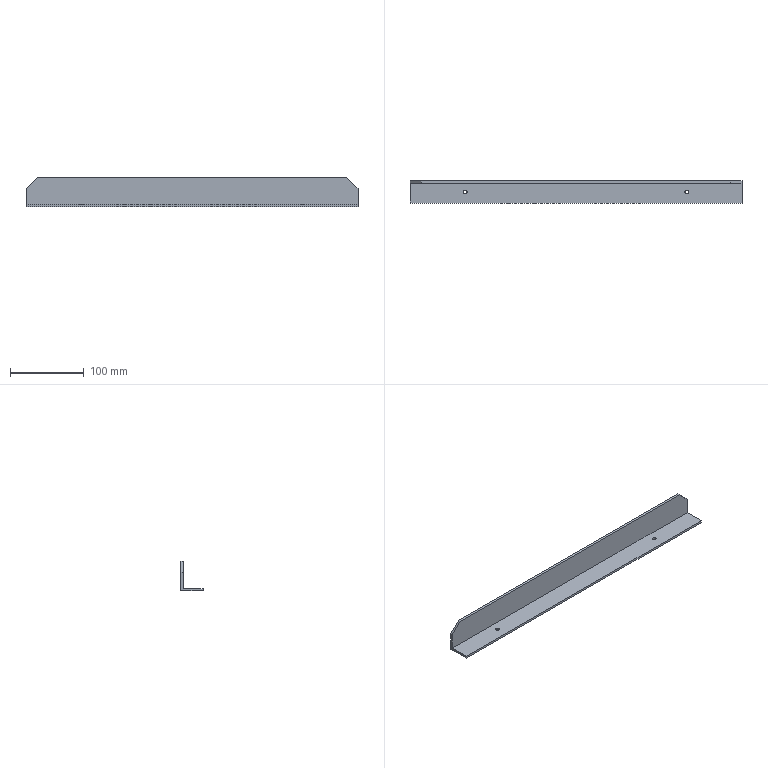Part | STEP file | Electrical cabinet partition strip | 1 solid | 14 faces | box 450 x 30 x 40 mm | volume 89657 mm3 | plane 10 | cylinder 4 | commonest cylinder face diameters 5 x4
STEP:
#1=CARTESIAN_POINT('',(0.,0.,0.));
#2=DIRECTION('',(0.,0.,1.));
#3=DIRECTION('',(1.,0.,0.));
#4=AXIS2_PLACEMENT_3D('',#1,#2,#3);
#5=CARTESIAN_POINT('',(77.5,30.066,-52.253));
#6=VERTEX_POINT('',#5);
#7=CARTESIAN_POINT('',(77.5,30.066,-49.253));
#8=VERTEX_POINT('',#7);
#9=CARTESIAN_POINT('',(77.5,30.066,-499.253));
#10=DIRECTION('',(0.,0.,1.));
#11=VECTOR('',#10,1.);
#12=LINE('',#9,#11);
#13=CARTESIAN_POINT('',(75.,30.066,-499.253));
#14=DIRECTION('',(0.,0.,1.));
#15=DIRECTION('',(1.,0.,0.));
#16=AXIS2_PLACEMENT_3D('',#13,#14,#15);
#17=CYLINDRICAL_SURFACE('',#16,2.5);
#18=CARTESIAN_POINT('',(6.283,0.));
#19=DIRECTION('',(0.,1.));
#20=VECTOR('',#19,1.);
#21=LINE('',#18,#20);
#22=(GEOMETRIC_REPRESENTATION_CONTEXT(2)PARAMETRIC_REPRESENTATION_CONTEXT()REPRESENTATION_CONTEXT('',''));
#23=DEFINITIONAL_REPRESENTATION('',(#21),#22);
#24=PCURVE('',#17,#23);
#25=CARTESIAN_POINT('',(75.,30.066,-499.253));
#26=DIRECTION('',(0.,0.,1.));
#27=DIRECTION('',(1.,0.,0.));
#28=AXIS2_PLACEMENT_3D('',#25,#26,#27);
#29=CYLINDRICAL_SURFACE('',#28,2.5);
#30=CARTESIAN_POINT('',(0.,0.));
#31=DIRECTION('',(0.,1.));
#32=VECTOR('',#31,1.);
#33=LINE('',#30,#32);
#34=(GEOMETRIC_REPRESENTATION_CONTEXT(2)PARAMETRIC_REPRESENTATION_CONTEXT()REPRESENTATION_CONTEXT('',''));
#35=DEFINITIONAL_REPRESENTATION('',(#33),#34);
#36=PCURVE('',#29,#35);
#37=SURFACE_CURVE('',#12,(#24,#36),.PCURVE_S1.);
#38=EDGE_CURVE('',#6,#8,#37,.T.);
#39=ORIENTED_EDGE('',*,*,#38,.T.);
#40=CARTESIAN_POINT('',(72.5,30.066,-49.253));
#41=VERTEX_POINT('',#40);
#42=CARTESIAN_POINT('',(75.,30.066,-49.253));
#43=DIRECTION('',(0.,0.,1.));
#44=DIRECTION('',(1.,0.,0.));
#45=AXIS2_PLACEMENT_3D('',#42,#43,#44);
#46=CIRCLE('',#45,2.5);
#47=CARTESIAN_POINT('',(0.,450.));
#48=DIRECTION('',(1.,0.));
#49=VECTOR('',#48,1.);
#50=LINE('',#47,#49);
#51=(GEOMETRIC_REPRESENTATION_CONTEXT(2)PARAMETRIC_REPRESENTATION_CONTEXT()REPRESENTATION_CONTEXT('',''));
#52=DEFINITIONAL_REPRESENTATION('',(#50),#51);
#53=PCURVE('',#17,#52);
#54=CARTESIAN_POINT('',(450.,42.066,-49.253));
#55=DIRECTION('',(0.,0.,-1.));
#56=DIRECTION('',(0.,1.,0.));
#57=AXIS2_PLACEMENT_3D('',#54,#55,#56);
#58=PLANE('',#57);
#59=CARTESIAN_POINT('',(-12.,-372.5));
#60=CARTESIAN_POINT('',(-7.67,-372.5));
#61=CARTESIAN_POINT('',(-9.835,-376.25));
#62=CARTESIAN_POINT('',(-12.,-380.));
#63=CARTESIAN_POINT('',(-14.165,-376.25));
#64=CARTESIAN_POINT('',(-16.33,-372.5));
#65=CARTESIAN_POINT('',(-12.,-372.5));
#66=(BOUNDED_CURVE()B_SPLINE_CURVE(2,(#59,#60,#61,#62,#63,#64,#65),.UNSPECIFIED.,.T.,.F.)B_SPLINE_CURVE_WITH_KNOTS((1,2,2,2,2,1),(-2.094,0.,2.094,4.189,6.283,8.378),.UNSPECIFIED.)CURVE()GEOMETRIC_REPRESENTATION_ITEM()RATIONAL_B_SPLINE_CURVE((1.,0.5,1.,0.5,1.,0.5,1.))REPRESENTATION_ITEM(''));
#67=(GEOMETRIC_REPRESENTATION_CONTEXT(2)PARAMETRIC_REPRESENTATION_CONTEXT()REPRESENTATION_CONTEXT('',''));
#68=DEFINITIONAL_REPRESENTATION('',(#66),#67);
#69=PCURVE('',#58,#68);
#70=SURFACE_CURVE('',#46,(#53,#69),.PCURVE_S1.);
#71=EDGE_CURVE('',#41,#8,#70,.T.);
#72=ORIENTED_EDGE('',*,*,#71,.F.);
#73=CARTESIAN_POINT('',(72.5,30.066,-52.253));
#74=VERTEX_POINT('',#73);
#75=CARTESIAN_POINT('',(72.5,30.066,-499.253));
#76=DIRECTION('',(0.,0.,1.));
#77=VECTOR('',#76,1.);
#78=LINE('',#75,#77);
#79=CARTESIAN_POINT('',(3.142,0.));
#80=DIRECTION('',(0.,1.));
#81=VECTOR('',#80,1.);
#82=LINE('',#79,#81);
#83=(GEOMETRIC_REPRESENTATION_CONTEXT(2)PARAMETRIC_REPRESENTATION_CONTEXT()REPRESENTATION_CONTEXT('',''));
#84=DEFINITIONAL_REPRESENTATION('',(#82),#83);
#85=PCURVE('',#17,#84);
#86=CARTESIAN_POINT('',(3.142,0.));
#87=DIRECTION('',(0.,1.));
#88=VECTOR('',#87,1.);
#89=LINE('',#86,#88);
#90=(GEOMETRIC_REPRESENTATION_CONTEXT(2)PARAMETRIC_REPRESENTATION_CONTEXT()REPRESENTATION_CONTEXT('',''));
#91=DEFINITIONAL_REPRESENTATION('',(#89),#90);
#92=PCURVE('',#29,#91);
#93=SURFACE_CURVE('',#78,(#85,#92),.PCURVE_S1.);
#94=EDGE_CURVE('',#74,#41,#93,.T.);
#95=ORIENTED_EDGE('',*,*,#94,.F.);
#96=CARTESIAN_POINT('',(75.,30.066,-52.253));
#97=DIRECTION('',(0.,0.,1.));
#98=DIRECTION('',(0.,-1.,0.));
#99=AXIS2_PLACEMENT_3D('',#96,#97,#98);
#100=CIRCLE('',#99,2.5);
#101=CARTESIAN_POINT('',(-1.571,447.));
#102=DIRECTION('',(1.,0.));
#103=VECTOR('',#102,1.);
#104=LINE('',#101,#103);
#105=(GEOMETRIC_REPRESENTATION_CONTEXT(2)PARAMETRIC_REPRESENTATION_CONTEXT()REPRESENTATION_CONTEXT('',''));
#106=DEFINITIONAL_REPRESENTATION('',(#104),#105);
#107=PCURVE('',#17,#106);
#108=CARTESIAN_POINT('',(450.,45.066,-52.253));
#109=DIRECTION('',(0.,0.,1.));
#110=DIRECTION('',(0.,-1.,0.));
#111=AXIS2_PLACEMENT_3D('',#108,#109,#110);
#112=PLANE('',#111);
#113=CARTESIAN_POINT('',(15.,-375.));
#114=DIRECTION('',(1.,0.));
#115=AXIS2_PLACEMENT_2D('',#113,#114);
#116=CIRCLE('',#115,2.5);
#117=(GEOMETRIC_REPRESENTATION_CONTEXT(2)PARAMETRIC_REPRESENTATION_CONTEXT()REPRESENTATION_CONTEXT('',''));
#118=DEFINITIONAL_REPRESENTATION('',(#116),#117);
#119=PCURVE('',#112,#118);
#120=SURFACE_CURVE('',#100,(#107,#119),.PCURVE_S1.);
#121=EDGE_CURVE('',#74,#6,#120,.T.);
#122=ORIENTED_EDGE('',*,*,#121,.T.);
#123=EDGE_LOOP('',(#39,#72,#95,#122));
#124=FACE_BOUND('',#123,.F.);
#125=ADVANCED_FACE('',(#124),#17,.F.);
#126=CARTESIAN_POINT('',(377.5,30.066,-52.253));
#127=VERTEX_POINT('',#126);
#128=CARTESIAN_POINT('',(377.5,30.066,-49.253));
#129=VERTEX_POINT('',#128);
#130=CARTESIAN_POINT('',(377.5,30.066,-499.253));
#131=DIRECTION('',(0.,0.,1.));
#132=VECTOR('',#131,1.);
#133=LINE('',#130,#132);
#134=CARTESIAN_POINT('',(375.,30.066,-499.253));
#135=DIRECTION('',(0.,0.,1.));
#136=DIRECTION('',(1.,0.,0.));
#137=AXIS2_PLACEMENT_3D('',#134,#135,#136);
#138=CYLINDRICAL_SURFACE('',#137,2.5);
#139=CARTESIAN_POINT('',(6.283,0.));
#140=DIRECTION('',(0.,1.));
#141=VECTOR('',#140,1.);
#142=LINE('',#139,#141);
#143=(GEOMETRIC_REPRESENTATION_CONTEXT(2)PARAMETRIC_REPRESENTATION_CONTEXT()REPRESENTATION_CONTEXT('',''));
#144=DEFINITIONAL_REPRESENTATION('',(#142),#143);
#145=PCURVE('',#138,#144);
#146=CARTESIAN_POINT('',(375.,30.066,-499.253));
#147=DIRECTION('',(0.,0.,1.));
#148=DIRECTION('',(1.,0.,0.));
#149=AXIS2_PLACEMENT_3D('',#146,#147,#148);
#150=CYLINDRICAL_SURFACE('',#149,2.5);
#151=CARTESIAN_POINT('',(0.,0.));
#152=DIRECTION('',(0.,1.));
#153=VECTOR('',#152,1.);
#154=LINE('',#151,#153);
#155=(GEOMETRIC_REPRESENTATION_CONTEXT(2)PARAMETRIC_REPRESENTATION_CONTEXT()REPRESENTATION_CONTEXT('',''));
#156=DEFINITIONAL_REPRESENTATION('',(#154),#155);
#157=PCURVE('',#150,#156);
#158=SURFACE_CURVE('',#133,(#145,#157),.PCURVE_S1.);
#159=EDGE_CURVE('',#127,#129,#158,.T.);
#160=ORIENTED_EDGE('',*,*,#159,.T.);
#161=CARTESIAN_POINT('',(372.5,30.066,-49.253));
#162=VERTEX_POINT('',#161);
#163=CARTESIAN_POINT('',(375.,30.066,-49.253));
#164=DIRECTION('',(0.,0.,1.));
#165=DIRECTION('',(1.,0.,0.));
#166=AXIS2_PLACEMENT_3D('',#163,#164,#165);
#167=CIRCLE('',#166,2.5);
#168=CARTESIAN_POINT('',(0.,450.));
#169=DIRECTION('',(1.,0.));
#170=VECTOR('',#169,1.);
#171=LINE('',#168,#170);
#172=(GEOMETRIC_REPRESENTATION_CONTEXT(2)PARAMETRIC_REPRESENTATION_CONTEXT()REPRESENTATION_CONTEXT('',''));
#173=DEFINITIONAL_REPRESENTATION('',(#171),#172);
#174=PCURVE('',#138,#173);
#175=CARTESIAN_POINT('',(-12.,-72.5));
#176=CARTESIAN_POINT('',(-7.67,-72.5));
#177=CARTESIAN_POINT('',(-9.835,-76.25));
#178=CARTESIAN_POINT('',(-12.,-80.));
#179=CARTESIAN_POINT('',(-14.165,-76.25));
#180=CARTESIAN_POINT('',(-16.33,-72.5));
#181=CARTESIAN_POINT('',(-12.,-72.5));
#182=(BOUNDED_CURVE()B_SPLINE_CURVE(2,(#175,#176,#177,#178,#179,#180,#181),.UNSPECIFIED.,.T.,.F.)B_SPLINE_CURVE_WITH_KNOTS((1,2,2,2,2,1),(-2.094,0.,2.094,4.189,6.283,8.378),.UNSPECIFIED.)CURVE()GEOMETRIC_REPRESENTATION_ITEM()RATIONAL_B_SPLINE_CURVE((1.,0.5,1.,0.5,1.,0.5,1.))REPRESENTATION_ITEM(''));
#183=(GEOMETRIC_REPRESENTATION_CONTEXT(2)PARAMETRIC_REPRESENTATION_CONTEXT()REPRESENTATION_CONTEXT('',''));
#184=DEFINITIONAL_REPRESENTATION('',(#182),#183);
#185=PCURVE('',#58,#184);
#186=SURFACE_CURVE('',#167,(#174,#185),.PCURVE_S1.);
#187=EDGE_CURVE('',#162,#129,#186,.T.);
#188=ORIENTED_EDGE('',*,*,#187,.F.);
#189=CARTESIAN_POINT('',(372.5,30.066,-52.253));
#190=VERTEX_POINT('',#189);
#191=CARTESIAN_POINT('',(372.5,30.066,-499.253));
#192=DIRECTION('',(0.,0.,1.));
#193=VECTOR('',#192,1.);
#194=LINE('',#191,#193);
#195=CARTESIAN_POINT('',(3.142,0.));
#196=DIRECTION('',(0.,1.));
#197=VECTOR('',#196,1.);
#198=LINE('',#195,#197);
#199=(GEOMETRIC_REPRESENTATION_CONTEXT(2)PARAMETRIC_REPRESENTATION_CONTEXT()REPRESENTATION_CONTEXT('',''));
#200=DEFINITIONAL_REPRESENTATION('',(#198),#199);
#201=PCURVE('',#138,#200);
#202=CARTESIAN_POINT('',(3.142,0.));
#203=DIRECTION('',(0.,1.));
#204=VECTOR('',#203,1.);
#205=LINE('',#202,#204);
#206=(GEOMETRIC_REPRESENTATION_CONTEXT(2)PARAMETRIC_REPRESENTATION_CONTEXT()REPRESENTATION_CONTEXT('',''));
#207=DEFINITIONAL_REPRESENTATION('',(#205),#206);
#208=PCURVE('',#150,#207);
#209=SURFACE_CURVE('',#194,(#201,#208),.PCURVE_S1.);
#210=EDGE_CURVE('',#190,#162,#209,.T.);
#211=ORIENTED_EDGE('',*,*,#210,.F.);
#212=CARTESIAN_POINT('',(375.,30.066,-52.253));
#213=DIRECTION('',(0.,0.,1.));
#214=DIRECTION('',(0.,-1.,0.));
#215=AXIS2_PLACEMENT_3D('',#212,#213,#214);
#216=CIRCLE('',#215,2.5);
#217=CARTESIAN_POINT('',(-1.571,447.));
#218=DIRECTION('',(1.,0.));
#219=VECTOR('',#218,1.);
#220=LINE('',#217,#219);
#221=(GEOMETRIC_REPRESENTATION_CONTEXT(2)PARAMETRIC_REPRESENTATION_CONTEXT()REPRESENTATION_CONTEXT('',''));
#222=DEFINITIONAL_REPRESENTATION('',(#220),#221);
#223=PCURVE('',#138,#222);
#224=CARTESIAN_POINT('',(15.,-75.));
#225=DIRECTION('',(1.,0.));
#226=AXIS2_PLACEMENT_2D('',#224,#225);
#227=CIRCLE('',#226,2.5);
#228=(GEOMETRIC_REPRESENTATION_CONTEXT(2)PARAMETRIC_REPRESENTATION_CONTEXT()REPRESENTATION_CONTEXT('',''));
#229=DEFINITIONAL_REPRESENTATION('',(#227),#228);
#230=PCURVE('',#112,#229);
#231=SURFACE_CURVE('',#216,(#223,#230),.PCURVE_S1.);
#232=EDGE_CURVE('',#190,#127,#231,.T.);
#233=ORIENTED_EDGE('',*,*,#232,.T.);
#234=EDGE_LOOP('',(#160,#188,#211,#233));
#235=FACE_BOUND('',#234,.F.);
#236=ADVANCED_FACE('',(#235),#138,.F.);
#237=CARTESIAN_POINT('',(435.,42.066,-12.253));
#238=VERTEX_POINT('',#237);
#239=CARTESIAN_POINT('',(15.,42.066,-12.253));
#240=VERTEX_POINT('',#239);
#241=CARTESIAN_POINT('',(450.,42.066,-12.253));
#242=DIRECTION('',(-1.,0.,0.));
#243=VECTOR('',#242,1.);
#244=LINE('',#241,#243);
#245=CARTESIAN_POINT('',(450.,42.066,-12.253));
#246=DIRECTION('',(0.,0.,-1.));
#247=DIRECTION('',(-1.,0.,0.));
#248=AXIS2_PLACEMENT_3D('',#245,#246,#247);
#249=PLANE('',#248);
#250=CARTESIAN_POINT('',(0.,0.));
#251=DIRECTION('',(1.,0.));
#252=VECTOR('',#251,1.);
#253=LINE('',#250,#252);
#254=(GEOMETRIC_REPRESENTATION_CONTEXT(2)PARAMETRIC_REPRESENTATION_CONTEXT()REPRESENTATION_CONTEXT('',''));
#255=DEFINITIONAL_REPRESENTATION('',(#253),#254);
#256=PCURVE('',#249,#255);
#257=CARTESIAN_POINT('',(450.,42.066,-12.253));
#258=DIRECTION('',(0.,1.,0.));
#259=DIRECTION('',(0.,0.,1.));
#260=AXIS2_PLACEMENT_3D('',#257,#258,#259);
#261=PLANE('',#260);
#262=CARTESIAN_POINT('',(0.,0.));
#263=DIRECTION('',(0.,-1.));
#264=VECTOR('',#263,1.);
#265=LINE('',#262,#264);
#266=(GEOMETRIC_REPRESENTATION_CONTEXT(2)PARAMETRIC_REPRESENTATION_CONTEXT()REPRESENTATION_CONTEXT('',''));
#267=DEFINITIONAL_REPRESENTATION('',(#265),#266);
#268=PCURVE('',#261,#267);
#269=SURFACE_CURVE('',#244,(#256,#268),.PCURVE_S1.);
#270=EDGE_CURVE('',#238,#240,#269,.T.);
#271=ORIENTED_EDGE('',*,*,#270,.F.);
#272=CARTESIAN_POINT('',(435.,45.066,-12.253));
#273=VERTEX_POINT('',#272);
#274=CARTESIAN_POINT('',(435.,42.066,-12.253));
#275=DIRECTION('',(0.,1.,0.));
#276=VECTOR('',#275,1.);
#277=LINE('',#274,#276);
#278=CARTESIAN_POINT('',(15.,0.));
#279=DIRECTION('',(0.,1.));
#280=VECTOR('',#279,1.);
#281=LINE('',#278,#280);
#282=(GEOMETRIC_REPRESENTATION_CONTEXT(2)PARAMETRIC_REPRESENTATION_CONTEXT()REPRESENTATION_CONTEXT('',''));
#283=DEFINITIONAL_REPRESENTATION('',(#281),#282);
#284=PCURVE('',#249,#283);
#285=CARTESIAN_POINT('',(450.,0.,-27.253));
#286=DIRECTION('',(-0.7071,0.,-0.7071));
#287=DIRECTION('',(0.,-1.,0.));
#288=AXIS2_PLACEMENT_3D('',#285,#286,#287);
#289=PLANE('',#288);
#290=CARTESIAN_POINT('',(-42.066,21.213));
#291=DIRECTION('',(-1.,0.));
#292=VECTOR('',#291,1.);
#293=LINE('',#290,#292);
#294=(GEOMETRIC_REPRESENTATION_CONTEXT(2)PARAMETRIC_REPRESENTATION_CONTEXT()REPRESENTATION_CONTEXT('',''));
#295=DEFINITIONAL_REPRESENTATION('',(#293),#294);
#296=PCURVE('',#289,#295);
#297=SURFACE_CURVE('',#277,(#284,#296),.PCURVE_S1.);
#298=EDGE_CURVE('',#238,#273,#297,.T.);
#299=ORIENTED_EDGE('',*,*,#298,.T.);
#300=CARTESIAN_POINT('',(15.,45.066,-12.253));
#301=VERTEX_POINT('',#300);
#302=CARTESIAN_POINT('',(450.,45.066,-12.253));
#303=DIRECTION('',(-1.,0.,0.));
#304=VECTOR('',#303,1.);
#305=LINE('',#302,#304);
#306=CARTESIAN_POINT('',(0.,3.));
#307=DIRECTION('',(1.,0.));
#308=VECTOR('',#307,1.);
#309=LINE('',#306,#308);
#310=(GEOMETRIC_REPRESENTATION_CONTEXT(2)PARAMETRIC_REPRESENTATION_CONTEXT()REPRESENTATION_CONTEXT('',''));
#311=DEFINITIONAL_REPRESENTATION('',(#309),#310);
#312=PCURVE('',#249,#311);
#313=CARTESIAN_POINT('',(450.,45.066,-12.253));
#314=DIRECTION('',(0.,-1.,0.));
#315=DIRECTION('',(0.,0.,-1.));
#316=AXIS2_PLACEMENT_3D('',#313,#314,#315);
#317=PLANE('',#316);
#318=CARTESIAN_POINT('',(0.,0.));
#319=DIRECTION('',(0.,-1.));
#320=VECTOR('',#319,1.);
#321=LINE('',#318,#320);
#322=(GEOMETRIC_REPRESENTATION_CONTEXT(2)PARAMETRIC_REPRESENTATION_CONTEXT()REPRESENTATION_CONTEXT('',''));
#323=DEFINITIONAL_REPRESENTATION('',(#321),#322);
#324=PCURVE('',#317,#323);
#325=SURFACE_CURVE('',#305,(#312,#324),.PCURVE_S1.);
#326=EDGE_CURVE('',#273,#301,#325,.T.);
#327=ORIENTED_EDGE('',*,*,#326,.T.);
#328=CARTESIAN_POINT('',(15.,42.066,-12.253));
#329=DIRECTION('',(0.,-1.,0.));
#330=VECTOR('',#329,1.);
#331=LINE('',#328,#330);
#332=CARTESIAN_POINT('',(435.,0.));
#333=DIRECTION('',(0.,-1.));
#334=VECTOR('',#333,1.);
#335=LINE('',#332,#334);
#336=(GEOMETRIC_REPRESENTATION_CONTEXT(2)PARAMETRIC_REPRESENTATION_CONTEXT()REPRESENTATION_CONTEXT('',''));
#337=DEFINITIONAL_REPRESENTATION('',(#335),#336);
#338=PCURVE('',#249,#337);
#339=CARTESIAN_POINT('',(15.,42.066,-12.253));
#340=DIRECTION('',(-0.7071,0.,0.7071));
#341=DIRECTION('',(0.,1.,0.));
#342=AXIS2_PLACEMENT_3D('',#339,#340,#341);
#343=PLANE('',#342);
#344=CARTESIAN_POINT('',(0.,0.));
#345=DIRECTION('',(-1.,0.));
#346=VECTOR('',#345,1.);
#347=LINE('',#344,#346);
#348=(GEOMETRIC_REPRESENTATION_CONTEXT(2)PARAMETRIC_REPRESENTATION_CONTEXT()REPRESENTATION_CONTEXT('',''));
#349=DEFINITIONAL_REPRESENTATION('',(#347),#348);
#350=PCURVE('',#343,#349);
#351=SURFACE_CURVE('',#331,(#338,#350),.PCURVE_S1.);
#352=EDGE_CURVE('',#301,#240,#351,.T.);
#353=ORIENTED_EDGE('',*,*,#352,.T.);
#354=EDGE_LOOP('',(#271,#299,#327,#353));
#355=FACE_BOUND('',#354,.T.);
#356=ADVANCED_FACE('',(#355),#249,.F.);
#357=CARTESIAN_POINT('',(450.,42.066,-27.253));
#358=VERTEX_POINT('',#357);
#359=CARTESIAN_POINT('',(450.,42.066,-49.253));
#360=VERTEX_POINT('',#359);
#361=CARTESIAN_POINT('',(450.,42.066,-12.253));
#362=DIRECTION('',(0.,0.,-1.));
#363=VECTOR('',#362,1.);
#364=LINE('',#361,#363);
#365=CARTESIAN_POINT('',(0.,0.));
#366=DIRECTION('',(-1.,0.));
#367=VECTOR('',#366,1.);
#368=LINE('',#365,#367);
#369=(GEOMETRIC_REPRESENTATION_CONTEXT(2)PARAMETRIC_REPRESENTATION_CONTEXT()REPRESENTATION_CONTEXT('',''));
#370=DEFINITIONAL_REPRESENTATION('',(#368),#369);
#371=PCURVE('',#261,#370);
#372=CARTESIAN_POINT('',(450.,0.,0.));
#373=DIRECTION('',(-1.,0.,0.));
#374=DIRECTION('',(0.,0.,1.));
#375=AXIS2_PLACEMENT_3D('',#372,#373,#374);
#376=PLANE('',#375);
#377=CARTESIAN_POINT('',(-12.253,42.066));
#378=DIRECTION('',(-1.,0.));
#379=VECTOR('',#378,1.);
#380=LINE('',#377,#379);
#381=(GEOMETRIC_REPRESENTATION_CONTEXT(2)PARAMETRIC_REPRESENTATION_CONTEXT()REPRESENTATION_CONTEXT('',''));
#382=DEFINITIONAL_REPRESENTATION('',(#380),#381);
#383=PCURVE('',#376,#382);
#384=SURFACE_CURVE('',#364,(#371,#383),.PCURVE_S1.);
#385=EDGE_CURVE('',#358,#360,#384,.T.);
#386=ORIENTED_EDGE('',*,*,#385,.F.);
#387=CARTESIAN_POINT('',(450.,42.066,-27.253));
#388=DIRECTION('',(-0.7071,0.,0.7071));
#389=VECTOR('',#388,1.);
#390=LINE('',#387,#389);
#391=CARTESIAN_POINT('',(-15.,0.));
#392=DIRECTION('',(0.7071,-0.7071));
#393=VECTOR('',#392,1.);
#394=LINE('',#391,#393);
#395=(GEOMETRIC_REPRESENTATION_CONTEXT(2)PARAMETRIC_REPRESENTATION_CONTEXT()REPRESENTATION_CONTEXT('',''));
#396=DEFINITIONAL_REPRESENTATION('',(#394),#395);
#397=PCURVE('',#261,#396);
#398=CARTESIAN_POINT('',(-42.066,0.));
#399=DIRECTION('',(0.,1.));
#400=VECTOR('',#399,1.);
#401=LINE('',#398,#400);
#402=(GEOMETRIC_REPRESENTATION_CONTEXT(2)PARAMETRIC_REPRESENTATION_CONTEXT()REPRESENTATION_CONTEXT('',''));
#403=DEFINITIONAL_REPRESENTATION('',(#401),#402);
#404=PCURVE('',#289,#403);
#405=SURFACE_CURVE('',#390,(#397,#404),.PCURVE_S1.);
#406=EDGE_CURVE('',#358,#238,#405,.T.);
#407=ORIENTED_EDGE('',*,*,#406,.T.);
#408=ORIENTED_EDGE('',*,*,#270,.T.);
#409=CARTESIAN_POINT('',(0.,42.066,-27.253));
#410=VERTEX_POINT('',#409);
#411=CARTESIAN_POINT('',(15.,42.066,-12.253));
#412=DIRECTION('',(-0.7071,0.,-0.7071));
#413=VECTOR('',#412,1.);
#414=LINE('',#411,#413);
#415=CARTESIAN_POINT('',(0.,-435.));
#416=DIRECTION('',(-0.7071,-0.7071));
#417=VECTOR('',#416,1.);
#418=LINE('',#415,#417);
#419=(GEOMETRIC_REPRESENTATION_CONTEXT(2)PARAMETRIC_REPRESENTATION_CONTEXT()REPRESENTATION_CONTEXT('',''));
#420=DEFINITIONAL_REPRESENTATION('',(#418),#419);
#421=PCURVE('',#261,#420);
#422=CARTESIAN_POINT('',(0.,0.));
#423=DIRECTION('',(0.,1.));
#424=VECTOR('',#423,1.);
#425=LINE('',#422,#424);
#426=(GEOMETRIC_REPRESENTATION_CONTEXT(2)PARAMETRIC_REPRESENTATION_CONTEXT()REPRESENTATION_CONTEXT('',''));
#427=DEFINITIONAL_REPRESENTATION('',(#425),#426);
#428=PCURVE('',#343,#427);
#429=SURFACE_CURVE('',#414,(#421,#428),.PCURVE_S1.);
#430=EDGE_CURVE('',#240,#410,#429,.T.);
#431=ORIENTED_EDGE('',*,*,#430,.T.);
#432=CARTESIAN_POINT('',(0.,42.066,-49.253));
#433=VERTEX_POINT('',#432);
#434=CARTESIAN_POINT('',(0.,42.066,-12.253));
#435=DIRECTION('',(0.,0.,-1.));
#436=VECTOR('',#435,1.);
#437=LINE('',#434,#436);
#438=CARTESIAN_POINT('',(0.,-450.));
#439=DIRECTION('',(-1.,0.));
#440=VECTOR('',#439,1.);
#441=LINE('',#438,#440);
#442=(GEOMETRIC_REPRESENTATION_CONTEXT(2)PARAMETRIC_REPRESENTATION_CONTEXT()REPRESENTATION_CONTEXT('',''));
#443=DEFINITIONAL_REPRESENTATION('',(#441),#442);
#444=PCURVE('',#261,#443);
#445=CARTESIAN_POINT('',(0.,0.,0.));
#446=DIRECTION('',(-1.,0.,0.));
#447=DIRECTION('',(0.,0.,1.));
#448=AXIS2_PLACEMENT_3D('',#445,#446,#447);
#449=PLANE('',#448);
#450=CARTESIAN_POINT('',(-12.253,42.066));
#451=DIRECTION('',(-1.,0.));
#452=VECTOR('',#451,1.);
#453=LINE('',#450,#452);
#454=(GEOMETRIC_REPRESENTATION_CONTEXT(2)PARAMETRIC_REPRESENTATION_CONTEXT()REPRESENTATION_CONTEXT('',''));
#455=DEFINITIONAL_REPRESENTATION('',(#453),#454);
#456=PCURVE('',#449,#455);
#457=SURFACE_CURVE('',#437,(#444,#456),.PCURVE_S1.);
#458=EDGE_CURVE('',#410,#433,#457,.T.);
#459=ORIENTED_EDGE('',*,*,#458,.T.);
#460=CARTESIAN_POINT('',(450.,42.066,-49.253));
#461=DIRECTION('',(-1.,0.,0.));
#462=VECTOR('',#461,1.);
#463=LINE('',#460,#462);
#464=CARTESIAN_POINT('',(-37.,0.));
#465=DIRECTION('',(0.,-1.));
#466=VECTOR('',#465,1.);
#467=LINE('',#464,#466);
#468=(GEOMETRIC_REPRESENTATION_CONTEXT(2)PARAMETRIC_REPRESENTATION_CONTEXT()REPRESENTATION_CONTEXT('',''));
#469=DEFINITIONAL_REPRESENTATION('',(#467),#468);
#470=PCURVE('',#261,#469);
#471=CARTESIAN_POINT('',(0.,0.));
#472=DIRECTION('',(0.,-1.));
#473=VECTOR('',#472,1.);
#474=LINE('',#471,#473);
#475=(GEOMETRIC_REPRESENTATION_CONTEXT(2)PARAMETRIC_REPRESENTATION_CONTEXT()REPRESENTATION_CONTEXT('',''));
#476=DEFINITIONAL_REPRESENTATION('',(#474),#475);
#477=PCURVE('',#58,#476);
#478=SURFACE_CURVE('',#463,(#470,#477),.PCURVE_S1.);
#479=EDGE_CURVE('',#360,#433,#478,.T.);
#480=ORIENTED_EDGE('',*,*,#479,.F.);
#481=EDGE_LOOP('',(#386,#407,#408,#431,#459,#480));
#482=FACE_BOUND('',#481,.T.);
#483=ADVANCED_FACE('',(#482),#261,.F.);
#484=CARTESIAN_POINT('',(75.,30.066,-49.253));
#485=DIRECTION('',(0.,0.,1.));
#486=DIRECTION('',(1.,0.,0.));
#487=AXIS2_PLACEMENT_3D('',#484,#485,#486);
#488=CIRCLE('',#487,2.5);
#489=CARTESIAN_POINT('',(-12.,-372.5));
#490=CARTESIAN_POINT('',(-7.67,-372.5));
#491=CARTESIAN_POINT('',(-9.835,-376.25));
#492=CARTESIAN_POINT('',(-12.,-380.));
#493=CARTESIAN_POINT('',(-14.165,-376.25));
#494=CARTESIAN_POINT('',(-16.33,-372.5));
#495=CARTESIAN_POINT('',(-12.,-372.5));
#496=(BOUNDED_CURVE()B_SPLINE_CURVE(2,(#489,#490,#491,#492,#493,#494,#495),.UNSPECIFIED.,.T.,.F.)B_SPLINE_CURVE_WITH_KNOTS((1,2,2,2,2,1),(-2.094,0.,2.094,4.189,6.283,8.378),.UNSPECIFIED.)CURVE()GEOMETRIC_REPRESENTATION_ITEM()RATIONAL_B_SPLINE_CURVE((1.,0.5,1.,0.5,1.,0.5,1.))REPRESENTATION_ITEM(''));
#497=(GEOMETRIC_REPRESENTATION_CONTEXT(2)PARAMETRIC_REPRESENTATION_CONTEXT()REPRESENTATION_CONTEXT('',''));
#498=DEFINITIONAL_REPRESENTATION('',(#496),#497);
#499=PCURVE('',#58,#498);
#500=CARTESIAN_POINT('',(0.,450.));
#501=DIRECTION('',(1.,0.));
#502=VECTOR('',#501,1.);
#503=LINE('',#500,#502);
#504=(GEOMETRIC_REPRESENTATION_CONTEXT(2)PARAMETRIC_REPRESENTATION_CONTEXT()REPRESENTATION_CONTEXT('',''));
#505=DEFINITIONAL_REPRESENTATION('',(#503),#504);
#506=PCURVE('',#29,#505);
#507=SURFACE_CURVE('',#488,(#499,#506),.PCURVE_S1.);
#508=EDGE_CURVE('',#8,#41,#507,.T.);
#509=ORIENTED_EDGE('',*,*,#508,.F.);
#510=ORIENTED_EDGE('',*,*,#71,.F.);
#511=EDGE_LOOP('',(#509,#510));
#512=FACE_BOUND('',#511,.T.);
#513=CARTESIAN_POINT('',(375.,30.066,-49.253));
#514=DIRECTION('',(0.,0.,1.));
#515=DIRECTION('',(1.,0.,0.));
#516=AXIS2_PLACEMENT_3D('',#513,#514,#515);
#517=CIRCLE('',#516,2.5);
#518=CARTESIAN_POINT('',(-12.,-72.5));
#519=CARTESIAN_POINT('',(-7.67,-72.5));
#520=CARTESIAN_POINT('',(-9.835,-76.25));
#521=CARTESIAN_POINT('',(-12.,-80.));
#522=CARTESIAN_POINT('',(-14.165,-76.25));
#523=CARTESIAN_POINT('',(-16.33,-72.5));
#524=CARTESIAN_POINT('',(-12.,-72.5));
#525=(BOUNDED_CURVE()B_SPLINE_CURVE(2,(#518,#519,#520,#521,#522,#523,#524),.UNSPECIFIED.,.T.,.F.)B_SPLINE_CURVE_WITH_KNOTS((1,2,2,2,2,1),(-2.094,0.,2.094,4.189,6.283,8.378),.UNSPECIFIED.)CURVE()GEOMETRIC_REPRESENTATION_ITEM()RATIONAL_B_SPLINE_CURVE((1.,0.5,1.,0.5,1.,0.5,1.))REPRESENTATION_ITEM(''));
#526=(GEOMETRIC_REPRESENTATION_CONTEXT(2)PARAMETRIC_REPRESENTATION_CONTEXT()REPRESENTATION_CONTEXT('',''));
#527=DEFINITIONAL_REPRESENTATION('',(#525),#526);
#528=PCURVE('',#58,#527);
#529=CARTESIAN_POINT('',(0.,450.));
#530=DIRECTION('',(1.,0.));
#531=VECTOR('',#530,1.);
#532=LINE('',#529,#531);
#533=(GEOMETRIC_REPRESENTATION_CONTEXT(2)PARAMETRIC_REPRESENTATION_CONTEXT()REPRESENTATION_CONTEXT('',''));
#534=DEFINITIONAL_REPRESENTATION('',(#532),#533);
#535=PCURVE('',#150,#534);
#536=SURFACE_CURVE('',#517,(#528,#535),.PCURVE_S1.);
#537=EDGE_CURVE('',#129,#162,#536,.T.);
#538=ORIENTED_EDGE('',*,*,#537,.F.);
#539=ORIENTED_EDGE('',*,*,#187,.F.);
#540=EDGE_LOOP('',(#538,#539));
#541=FACE_BOUND('',#540,.T.);
#542=CARTESIAN_POINT('',(0.,15.066,-49.253));
#543=VERTEX_POINT('',#542);
#544=CARTESIAN_POINT('',(0.,42.066,-49.253));
#545=DIRECTION('',(0.,-1.,0.));
#546=VECTOR('',#545,1.);
#547=LINE('',#544,#546);
#548=CARTESIAN_POINT('',(0.,-450.));
#549=DIRECTION('',(-1.,0.));
#550=VECTOR('',#549,1.);
#551=LINE('',#548,#550);
#552=(GEOMETRIC_REPRESENTATION_CONTEXT(2)PARAMETRIC_REPRESENTATION_CONTEXT()REPRESENTATION_CONTEXT('',''));
#553=DEFINITIONAL_REPRESENTATION('',(#551),#552);
#554=PCURVE('',#58,#553);
#555=CARTESIAN_POINT('',(-49.253,42.066));
#556=DIRECTION('',(0.,-1.));
#557=VECTOR('',#556,1.);
#558=LINE('',#555,#557);
#559=(GEOMETRIC_REPRESENTATION_CONTEXT(2)PARAMETRIC_REPRESENTATION_CONTEXT()REPRESENTATION_CONTEXT('',''));
#560=DEFINITIONAL_REPRESENTATION('',(#558),#559);
#561=PCURVE('',#449,#560);
#562=SURFACE_CURVE('',#547,(#554,#561),.PCURVE_S1.);
#563=EDGE_CURVE('',#433,#543,#562,.T.);
#564=ORIENTED_EDGE('',*,*,#563,.T.);
#565=CARTESIAN_POINT('',(450.,15.066,-49.253));
#566=VERTEX_POINT('',#565);
#567=CARTESIAN_POINT('',(450.,15.066,-49.253));
#568=DIRECTION('',(-1.,0.,0.));
#569=VECTOR('',#568,1.);
#570=LINE('',#567,#569);
#571=CARTESIAN_POINT('',(-27.,0.));
#572=DIRECTION('',(0.,-1.));
#573=VECTOR('',#572,1.);
#574=LINE('',#571,#573);
#575=(GEOMETRIC_REPRESENTATION_CONTEXT(2)PARAMETRIC_REPRESENTATION_CONTEXT()REPRESENTATION_CONTEXT('',''));
#576=DEFINITIONAL_REPRESENTATION('',(#574),#575);
#577=PCURVE('',#58,#576);
#578=CARTESIAN_POINT('',(450.,15.066,-49.253));
#579=DIRECTION('',(0.,1.,0.));
#580=DIRECTION('',(0.,0.,1.));
#581=AXIS2_PLACEMENT_3D('',#578,#579,#580);
#582=PLANE('',#581);
#583=CARTESIAN_POINT('',(0.,0.));
#584=DIRECTION('',(0.,-1.));
#585=VECTOR('',#584,1.);
#586=LINE('',#583,#585);
#587=(GEOMETRIC_REPRESENTATION_CONTEXT(2)PARAMETRIC_REPRESENTATION_CONTEXT()REPRESENTATION_CONTEXT('',''));
#588=DEFINITIONAL_REPRESENTATION('',(#586),#587);
#589=PCURVE('',#582,#588);
#590=SURFACE_CURVE('',#570,(#577,#589),.PCURVE_S1.);
#591=EDGE_CURVE('',#566,#543,#590,.T.);
#592=ORIENTED_EDGE('',*,*,#591,.F.);
#593=CARTESIAN_POINT('',(450.,42.066,-49.253));
#594=DIRECTION('',(0.,-1.,0.));
#595=VECTOR('',#594,1.);
#596=LINE('',#593,#595);
#597=CARTESIAN_POINT('',(0.,0.));
#598=DIRECTION('',(-1.,0.));
#599=VECTOR('',#598,1.);
#600=LINE('',#597,#599);
#601=(GEOMETRIC_REPRESENTATION_CONTEXT(2)PARAMETRIC_REPRESENTATION_CONTEXT()REPRESENTATION_CONTEXT('',''));
#602=DEFINITIONAL_REPRESENTATION('',(#600),#601);
#603=PCURVE('',#58,#602);
#604=CARTESIAN_POINT('',(-49.253,42.066));
#605=DIRECTION('',(0.,-1.));
#606=VECTOR('',#605,1.);
#607=LINE('',#604,#606);
#608=(GEOMETRIC_REPRESENTATION_CONTEXT(2)PARAMETRIC_REPRESENTATION_CONTEXT()REPRESENTATION_CONTEXT('',''));
#609=DEFINITIONAL_REPRESENTATION('',(#607),#608);
#610=PCURVE('',#376,#609);
#611=SURFACE_CURVE('',#596,(#603,#610),.PCURVE_S1.);
#612=EDGE_CURVE('',#360,#566,#611,.T.);
#613=ORIENTED_EDGE('',*,*,#612,.F.);
#614=ORIENTED_EDGE('',*,*,#479,.T.);
#615=EDGE_LOOP('',(#564,#592,#613,#614));
#616=FACE_BOUND('',#615,.T.);
#617=ADVANCED_FACE('',(#512,#541,#616),#58,.F.);
#618=CARTESIAN_POINT('',(0.,15.066,-52.253));
#619=VERTEX_POINT('',#618);
#620=CARTESIAN_POINT('',(0.,15.066,-49.253));
#621=DIRECTION('',(0.,0.,-1.));
#622=VECTOR('',#621,1.);
#623=LINE('',#620,#622);
#624=CARTESIAN_POINT('',(0.,-450.));
#625=DIRECTION('',(-1.,0.));
#626=VECTOR('',#625,1.);
#627=LINE('',#624,#626);
#628=(GEOMETRIC_REPRESENTATION_CONTEXT(2)PARAMETRIC_REPRESENTATION_CONTEXT()REPRESENTATION_CONTEXT('',''));
#629=DEFINITIONAL_REPRESENTATION('',(#627),#628);
#630=PCURVE('',#582,#629);
#631=CARTESIAN_POINT('',(-49.253,15.066));
#632=DIRECTION('',(-1.,0.));
#633=VECTOR('',#632,1.);
#634=LINE('',#631,#633);
#635=(GEOMETRIC_REPRESENTATION_CONTEXT(2)PARAMETRIC_REPRESENTATION_CONTEXT()REPRESENTATION_CONTEXT('',''));
#636=DEFINITIONAL_REPRESENTATION('',(#634),#635);
#637=PCURVE('',#449,#636);
#638=SURFACE_CURVE('',#623,(#630,#637),.PCURVE_S1.);
#639=EDGE_CURVE('',#543,#619,#638,.T.);
#640=ORIENTED_EDGE('',*,*,#639,.T.);
#641=CARTESIAN_POINT('',(450.,15.066,-52.253));
#642=VERTEX_POINT('',#641);
#643=CARTESIAN_POINT('',(450.,15.066,-52.253));
#644=DIRECTION('',(-1.,0.,0.));
#645=VECTOR('',#644,1.);
#646=LINE('',#643,#645);
#647=CARTESIAN_POINT('',(-3.,0.));
#648=DIRECTION('',(0.,-1.));
#649=VECTOR('',#648,1.);
#650=LINE('',#647,#649);
#651=(GEOMETRIC_REPRESENTATION_CONTEXT(2)PARAMETRIC_REPRESENTATION_CONTEXT()REPRESENTATION_CONTEXT('',''));
#652=DEFINITIONAL_REPRESENTATION('',(#650),#651);
#653=PCURVE('',#582,#652);
#654=CARTESIAN_POINT('',(30.,0.));
#655=DIRECTION('',(0.,-1.));
#656=VECTOR('',#655,1.);
#657=LINE('',#654,#656);
#658=(GEOMETRIC_REPRESENTATION_CONTEXT(2)PARAMETRIC_REPRESENTATION_CONTEXT()REPRESENTATION_CONTEXT('',''));
#659=DEFINITIONAL_REPRESENTATION('',(#657),#658);
#660=PCURVE('',#112,#659);
#661=SURFACE_CURVE('',#646,(#653,#660),.PCURVE_S1.);
#662=EDGE_CURVE('',#642,#619,#661,.T.);
#663=ORIENTED_EDGE('',*,*,#662,.F.);
#664=CARTESIAN_POINT('',(450.,15.066,-49.253));
#665=DIRECTION('',(0.,0.,-1.));
#666=VECTOR('',#665,1.);
#667=LINE('',#664,#666);
#668=CARTESIAN_POINT('',(0.,0.));
#669=DIRECTION('',(-1.,0.));
#670=VECTOR('',#669,1.);
#671=LINE('',#668,#670);
#672=(GEOMETRIC_REPRESENTATION_CONTEXT(2)PARAMETRIC_REPRESENTATION_CONTEXT()REPRESENTATION_CONTEXT('',''));
#673=DEFINITIONAL_REPRESENTATION('',(#671),#672);
#674=PCURVE('',#582,#673);
#675=CARTESIAN_POINT('',(-49.253,15.066));
#676=DIRECTION('',(-1.,0.));
#677=VECTOR('',#676,1.);
#678=LINE('',#675,#677);
#679=(GEOMETRIC_REPRESENTATION_CONTEXT(2)PARAMETRIC_REPRESENTATION_CONTEXT()REPRESENTATION_CONTEXT('',''));
#680=DEFINITIONAL_REPRESENTATION('',(#678),#679);
#681=PCURVE('',#376,#680);
#682=SURFACE_CURVE('',#667,(#674,#681),.PCURVE_S1.);
#683=EDGE_CURVE('',#566,#642,#682,.T.);
#684=ORIENTED_EDGE('',*,*,#683,.F.);
#685=ORIENTED_EDGE('',*,*,#591,.T.);
#686=EDGE_LOOP('',(#640,#663,#684,#685));
#687=FACE_BOUND('',#686,.T.);
#688=ADVANCED_FACE('',(#687),#582,.F.);
#689=CARTESIAN_POINT('',(75.,30.066,-52.253));
#690=DIRECTION('',(0.,0.,1.));
#691=DIRECTION('',(0.,-1.,0.));
#692=AXIS2_PLACEMENT_3D('',#689,#690,#691);
#693=CIRCLE('',#692,2.5);
#694=CARTESIAN_POINT('',(15.,-375.));
#695=DIRECTION('',(1.,0.));
#696=AXIS2_PLACEMENT_2D('',#694,#695);
#697=CIRCLE('',#696,2.5);
#698=(GEOMETRIC_REPRESENTATION_CONTEXT(2)PARAMETRIC_REPRESENTATION_CONTEXT()REPRESENTATION_CONTEXT('',''));
#699=DEFINITIONAL_REPRESENTATION('',(#697),#698);
#700=PCURVE('',#112,#699);
#701=CARTESIAN_POINT('',(-1.571,447.));
#702=DIRECTION('',(1.,0.));
#703=VECTOR('',#702,1.);
#704=LINE('',#701,#703);
#705=(GEOMETRIC_REPRESENTATION_CONTEXT(2)PARAMETRIC_REPRESENTATION_CONTEXT()REPRESENTATION_CONTEXT('',''));
#706=DEFINITIONAL_REPRESENTATION('',(#704),#705);
#707=PCURVE('',#29,#706);
#708=SURFACE_CURVE('',#693,(#700,#707),.PCURVE_S1.);
#709=EDGE_CURVE('',#6,#74,#708,.T.);
#710=ORIENTED_EDGE('',*,*,#709,.T.);
#711=ORIENTED_EDGE('',*,*,#121,.T.);
#712=EDGE_LOOP('',(#710,#711));
#713=FACE_BOUND('',#712,.T.);
#714=CARTESIAN_POINT('',(375.,30.066,-52.253));
#715=DIRECTION('',(0.,0.,1.));
#716=DIRECTION('',(0.,-1.,0.));
#717=AXIS2_PLACEMENT_3D('',#714,#715,#716);
#718=CIRCLE('',#717,2.5);
#719=CARTESIAN_POINT('',(15.,-75.));
#720=DIRECTION('',(1.,0.));
#721=AXIS2_PLACEMENT_2D('',#719,#720);
#722=CIRCLE('',#721,2.5);
#723=(GEOMETRIC_REPRESENTATION_CONTEXT(2)PARAMETRIC_REPRESENTATION_CONTEXT()REPRESENTATION_CONTEXT('',''));
#724=DEFINITIONAL_REPRESENTATION('',(#722),#723);
#725=PCURVE('',#112,#724);
#726=CARTESIAN_POINT('',(-1.571,447.));
#727=DIRECTION('',(1.,0.));
#728=VECTOR('',#727,1.);
#729=LINE('',#726,#728);
#730=(GEOMETRIC_REPRESENTATION_CONTEXT(2)PARAMETRIC_REPRESENTATION_CONTEXT()REPRESENTATION_CONTEXT('',''));
#731=DEFINITIONAL_REPRESENTATION('',(#729),#730);
#732=PCURVE('',#150,#731);
#733=SURFACE_CURVE('',#718,(#725,#732),.PCURVE_S1.);
#734=EDGE_CURVE('',#127,#190,#733,.T.);
#735=ORIENTED_EDGE('',*,*,#734,.T.);
#736=ORIENTED_EDGE('',*,*,#232,.T.);
#737=EDGE_LOOP('',(#735,#736));
#738=FACE_BOUND('',#737,.T.);
#739=CARTESIAN_POINT('',(0.,45.066,-52.253));
#740=VERTEX_POINT('',#739);
#741=CARTESIAN_POINT('',(0.,45.066,-52.253));
#742=DIRECTION('',(0.,1.,0.));
#743=VECTOR('',#742,1.);
#744=LINE('',#741,#743);
#745=CARTESIAN_POINT('',(0.,-450.));
#746=DIRECTION('',(-1.,0.));
#747=VECTOR('',#746,1.);
#748=LINE('',#745,#747);
#749=(GEOMETRIC_REPRESENTATION_CONTEXT(2)PARAMETRIC_REPRESENTATION_CONTEXT()REPRESENTATION_CONTEXT('',''));
#750=DEFINITIONAL_REPRESENTATION('',(#748),#749);
#751=PCURVE('',#112,#750);
#752=CARTESIAN_POINT('',(-52.253,45.066));
#753=DIRECTION('',(0.,1.));
#754=VECTOR('',#753,1.);
#755=LINE('',#752,#754);
#756=(GEOMETRIC_REPRESENTATION_CONTEXT(2)PARAMETRIC_REPRESENTATION_CONTEXT()REPRESENTATION_CONTEXT('',''));
#757=DEFINITIONAL_REPRESENTATION('',(#755),#756);
#758=PCURVE('',#449,#757);
#759=SURFACE_CURVE('',#744,(#751,#758),.PCURVE_S1.);
#760=EDGE_CURVE('',#619,#740,#759,.T.);
#761=ORIENTED_EDGE('',*,*,#760,.T.);
#762=CARTESIAN_POINT('',(450.,45.066,-52.253));
#763=VERTEX_POINT('',#762);
#764=CARTESIAN_POINT('',(450.,45.066,-52.253));
#765=DIRECTION('',(-1.,0.,0.));
#766=VECTOR('',#765,1.);
#767=LINE('',#764,#766);
#768=CARTESIAN_POINT('',(0.,0.));
#769=DIRECTION('',(0.,-1.));
#770=VECTOR('',#769,1.);
#771=LINE('',#768,#770);
#772=(GEOMETRIC_REPRESENTATION_CONTEXT(2)PARAMETRIC_REPRESENTATION_CONTEXT()REPRESENTATION_CONTEXT('',''));
#773=DEFINITIONAL_REPRESENTATION('',(#771),#772);
#774=PCURVE('',#112,#773);
#775=CARTESIAN_POINT('',(40.,0.));
#776=DIRECTION('',(0.,-1.));
#777=VECTOR('',#776,1.);
#778=LINE('',#775,#777);
#779=(GEOMETRIC_REPRESENTATION_CONTEXT(2)PARAMETRIC_REPRESENTATION_CONTEXT()REPRESENTATION_CONTEXT('',''));
#780=DEFINITIONAL_REPRESENTATION('',(#778),#779);
#781=PCURVE('',#317,#780);
#782=SURFACE_CURVE('',#767,(#774,#781),.PCURVE_S1.);
#783=EDGE_CURVE('',#763,#740,#782,.T.);
#784=ORIENTED_EDGE('',*,*,#783,.F.);
#785=CARTESIAN_POINT('',(450.,45.066,-52.253));
#786=DIRECTION('',(0.,1.,0.));
#787=VECTOR('',#786,1.);
#788=LINE('',#785,#787);
#789=CARTESIAN_POINT('',(0.,0.));
#790=DIRECTION('',(-1.,0.));
#791=VECTOR('',#790,1.);
#792=LINE('',#789,#791);
#793=(GEOMETRIC_REPRESENTATION_CONTEXT(2)PARAMETRIC_REPRESENTATION_CONTEXT()REPRESENTATION_CONTEXT('',''));
#794=DEFINITIONAL_REPRESENTATION('',(#792),#793);
#795=PCURVE('',#112,#794);
#796=CARTESIAN_POINT('',(-52.253,45.066));
#797=DIRECTION('',(0.,1.));
#798=VECTOR('',#797,1.);
#799=LINE('',#796,#798);
#800=(GEOMETRIC_REPRESENTATION_CONTEXT(2)PARAMETRIC_REPRESENTATION_CONTEXT()REPRESENTATION_CONTEXT('',''));
#801=DEFINITIONAL_REPRESENTATION('',(#799),#800);
#802=PCURVE('',#376,#801);
#803=SURFACE_CURVE('',#788,(#795,#802),.PCURVE_S1.);
#804=EDGE_CURVE('',#642,#763,#803,.T.);
#805=ORIENTED_EDGE('',*,*,#804,.F.);
#806=ORIENTED_EDGE('',*,*,#662,.T.);
#807=EDGE_LOOP('',(#761,#784,#805,#806));
#808=FACE_BOUND('',#807,.T.);
#809=ADVANCED_FACE('',(#713,#738,#808),#112,.F.);
#810=ORIENTED_EDGE('',*,*,#326,.F.);
#811=CARTESIAN_POINT('',(450.,45.066,-27.253));
#812=VERTEX_POINT('',#811);
#813=CARTESIAN_POINT('',(450.,45.066,-27.253));
#814=DIRECTION('',(0.7071,0.,-0.7071));
#815=VECTOR('',#814,1.);
#816=LINE('',#813,#815);
#817=CARTESIAN_POINT('',(15.,0.));
#818=DIRECTION('',(0.7071,0.7071));
#819=VECTOR('',#818,1.);
#820=LINE('',#817,#819);
#821=(GEOMETRIC_REPRESENTATION_CONTEXT(2)PARAMETRIC_REPRESENTATION_CONTEXT()REPRESENTATION_CONTEXT('',''));
#822=DEFINITIONAL_REPRESENTATION('',(#820),#821);
#823=PCURVE('',#317,#822);
#824=CARTESIAN_POINT('',(-45.066,0.));
#825=DIRECTION('',(0.,-1.));
#826=VECTOR('',#825,1.);
#827=LINE('',#824,#826);
#828=(GEOMETRIC_REPRESENTATION_CONTEXT(2)PARAMETRIC_REPRESENTATION_CONTEXT()REPRESENTATION_CONTEXT('',''));
#829=DEFINITIONAL_REPRESENTATION('',(#827),#828);
#830=PCURVE('',#289,#829);
#831=SURFACE_CURVE('',#816,(#823,#830),.PCURVE_S1.);
#832=EDGE_CURVE('',#273,#812,#831,.T.);
#833=ORIENTED_EDGE('',*,*,#832,.T.);
#834=CARTESIAN_POINT('',(450.,45.066,-12.253));
#835=DIRECTION('',(0.,0.,1.));
#836=VECTOR('',#835,1.);
#837=LINE('',#834,#836);
#838=CARTESIAN_POINT('',(0.,0.));
#839=DIRECTION('',(-1.,0.));
#840=VECTOR('',#839,1.);
#841=LINE('',#838,#840);
#842=(GEOMETRIC_REPRESENTATION_CONTEXT(2)PARAMETRIC_REPRESENTATION_CONTEXT()REPRESENTATION_CONTEXT('',''));
#843=DEFINITIONAL_REPRESENTATION('',(#841),#842);
#844=PCURVE('',#317,#843);
#845=CARTESIAN_POINT('',(-12.253,45.066));
#846=DIRECTION('',(1.,0.));
#847=VECTOR('',#846,1.);
#848=LINE('',#845,#847);
#849=(GEOMETRIC_REPRESENTATION_CONTEXT(2)PARAMETRIC_REPRESENTATION_CONTEXT()REPRESENTATION_CONTEXT('',''));
#850=DEFINITIONAL_REPRESENTATION('',(#848),#849);
#851=PCURVE('',#376,#850);
#852=SURFACE_CURVE('',#837,(#844,#851),.PCURVE_S1.);
#853=EDGE_CURVE('',#763,#812,#852,.T.);
#854=ORIENTED_EDGE('',*,*,#853,.F.);
#855=ORIENTED_EDGE('',*,*,#783,.T.);
#856=CARTESIAN_POINT('',(0.,45.066,-27.253));
#857=VERTEX_POINT('',#856);
#858=CARTESIAN_POINT('',(0.,45.066,-12.253));
#859=DIRECTION('',(0.,0.,1.));
#860=VECTOR('',#859,1.);
#861=LINE('',#858,#860);
#862=CARTESIAN_POINT('',(0.,-450.));
#863=DIRECTION('',(-1.,0.));
#864=VECTOR('',#863,1.);
#865=LINE('',#862,#864);
#866=(GEOMETRIC_REPRESENTATION_CONTEXT(2)PARAMETRIC_REPRESENTATION_CONTEXT()REPRESENTATION_CONTEXT('',''));
#867=DEFINITIONAL_REPRESENTATION('',(#865),#866);
#868=PCURVE('',#317,#867);
#869=CARTESIAN_POINT('',(-12.253,45.066));
#870=DIRECTION('',(1.,0.));
#871=VECTOR('',#870,1.);
#872=LINE('',#869,#871);
#873=(GEOMETRIC_REPRESENTATION_CONTEXT(2)PARAMETRIC_REPRESENTATION_CONTEXT()REPRESENTATION_CONTEXT('',''));
#874=DEFINITIONAL_REPRESENTATION('',(#872),#873);
#875=PCURVE('',#449,#874);
#876=SURFACE_CURVE('',#861,(#868,#875),.PCURVE_S1.);
#877=EDGE_CURVE('',#740,#857,#876,.T.);
#878=ORIENTED_EDGE('',*,*,#877,.T.);
#879=CARTESIAN_POINT('',(15.,45.066,-12.253));
#880=DIRECTION('',(0.7071,0.,0.7071));
#881=VECTOR('',#880,1.);
#882=LINE('',#879,#881);
#883=CARTESIAN_POINT('',(0.,-435.));
#884=DIRECTION('',(-0.7071,0.7071));
#885=VECTOR('',#884,1.);
#886=LINE('',#883,#885);
#887=(GEOMETRIC_REPRESENTATION_CONTEXT(2)PARAMETRIC_REPRESENTATION_CONTEXT()REPRESENTATION_CONTEXT('',''));
#888=DEFINITIONAL_REPRESENTATION('',(#886),#887);
#889=PCURVE('',#317,#888);
#890=CARTESIAN_POINT('',(3.,0.));
#891=DIRECTION('',(0.,-1.));
#892=VECTOR('',#891,1.);
#893=LINE('',#890,#892);
#894=(GEOMETRIC_REPRESENTATION_CONTEXT(2)PARAMETRIC_REPRESENTATION_CONTEXT()REPRESENTATION_CONTEXT('',''));
#895=DEFINITIONAL_REPRESENTATION('',(#893),#894);
#896=PCURVE('',#343,#895);
#897=SURFACE_CURVE('',#882,(#889,#896),.PCURVE_S1.);
#898=EDGE_CURVE('',#857,#301,#897,.T.);
#899=ORIENTED_EDGE('',*,*,#898,.T.);
#900=EDGE_LOOP('',(#810,#833,#854,#855,#878,#899));
#901=FACE_BOUND('',#900,.T.);
#902=ADVANCED_FACE('',(#901),#317,.F.);
#903=ORIENTED_EDGE('',*,*,#853,.T.);
#904=CARTESIAN_POINT('',(450.,0.,-27.253));
#905=DIRECTION('',(0.,-1.,0.));
#906=VECTOR('',#905,1.);
#907=LINE('',#904,#906);
#908=CARTESIAN_POINT('',(-27.253,0.));
#909=DIRECTION('',(0.,-1.));
#910=VECTOR('',#909,1.);
#911=LINE('',#908,#910);
#912=(GEOMETRIC_REPRESENTATION_CONTEXT(2)PARAMETRIC_REPRESENTATION_CONTEXT()REPRESENTATION_CONTEXT('',''));
#913=DEFINITIONAL_REPRESENTATION('',(#911),#912);
#914=PCURVE('',#376,#913);
#915=CARTESIAN_POINT('',(0.,0.));
#916=DIRECTION('',(1.,0.));
#917=VECTOR('',#916,1.);
#918=LINE('',#915,#917);
#919=(GEOMETRIC_REPRESENTATION_CONTEXT(2)PARAMETRIC_REPRESENTATION_CONTEXT()REPRESENTATION_CONTEXT('',''));
#920=DEFINITIONAL_REPRESENTATION('',(#918),#919);
#921=PCURVE('',#289,#920);
#922=SURFACE_CURVE('',#907,(#914,#921),.PCURVE_S1.);
#923=EDGE_CURVE('',#812,#358,#922,.T.);
#924=ORIENTED_EDGE('',*,*,#923,.T.);
#925=ORIENTED_EDGE('',*,*,#385,.T.);
#926=ORIENTED_EDGE('',*,*,#612,.T.);
#927=ORIENTED_EDGE('',*,*,#683,.T.);
#928=ORIENTED_EDGE('',*,*,#804,.T.);
#929=EDGE_LOOP('',(#903,#924,#925,#926,#927,#928));
#930=FACE_BOUND('',#929,.T.);
#931=ADVANCED_FACE('',(#930),#376,.F.);
#932=ORIENTED_EDGE('',*,*,#458,.F.);
#933=CARTESIAN_POINT('',(0.,45.066,-27.253));
#934=DIRECTION('',(0.,1.,0.));
#935=VECTOR('',#934,1.);
#936=LINE('',#933,#935);
#937=CARTESIAN_POINT('',(-27.253,45.066));
#938=DIRECTION('',(0.,1.));
#939=VECTOR('',#938,1.);
#940=LINE('',#937,#939);
#941=(GEOMETRIC_REPRESENTATION_CONTEXT(2)PARAMETRIC_REPRESENTATION_CONTEXT()REPRESENTATION_CONTEXT('',''));
#942=DEFINITIONAL_REPRESENTATION('',(#940),#941);
#943=PCURVE('',#449,#942);
#944=CARTESIAN_POINT('',(3.,21.213));
#945=DIRECTION('',(1.,0.));
#946=VECTOR('',#945,1.);
#947=LINE('',#944,#946);
#948=(GEOMETRIC_REPRESENTATION_CONTEXT(2)PARAMETRIC_REPRESENTATION_CONTEXT()REPRESENTATION_CONTEXT('',''));
#949=DEFINITIONAL_REPRESENTATION('',(#947),#948);
#950=PCURVE('',#343,#949);
#951=SURFACE_CURVE('',#936,(#943,#950),.PCURVE_S1.);
#952=EDGE_CURVE('',#410,#857,#951,.T.);
#953=ORIENTED_EDGE('',*,*,#952,.T.);
#954=ORIENTED_EDGE('',*,*,#877,.F.);
#955=ORIENTED_EDGE('',*,*,#760,.F.);
#956=ORIENTED_EDGE('',*,*,#639,.F.);
#957=ORIENTED_EDGE('',*,*,#563,.F.);
#958=EDGE_LOOP('',(#932,#953,#954,#955,#956,#957));
#959=FACE_BOUND('',#958,.T.);
#960=ADVANCED_FACE('',(#959),#449,.T.);
#961=ORIENTED_EDGE('',*,*,#537,.F.);
#962=ORIENTED_EDGE('',*,*,#159,.F.);
#963=ORIENTED_EDGE('',*,*,#734,.T.);
#964=ORIENTED_EDGE('',*,*,#210,.T.);
#965=EDGE_LOOP('',(#961,#962,#963,#964));
#966=FACE_BOUND('',#965,.F.);
#967=ADVANCED_FACE('',(#966),#150,.F.);
#968=ORIENTED_EDGE('',*,*,#508,.F.);
#969=ORIENTED_EDGE('',*,*,#38,.F.);
#970=ORIENTED_EDGE('',*,*,#709,.T.);
#971=ORIENTED_EDGE('',*,*,#94,.T.);
#972=EDGE_LOOP('',(#968,#969,#970,#971));
#973=FACE_BOUND('',#972,.F.);
#974=ADVANCED_FACE('',(#973),#29,.F.);
#975=ORIENTED_EDGE('',*,*,#832,.F.);
#976=ORIENTED_EDGE('',*,*,#298,.F.);
#977=ORIENTED_EDGE('',*,*,#406,.F.);
#978=ORIENTED_EDGE('',*,*,#923,.F.);
#979=EDGE_LOOP('',(#975,#976,#977,#978));
#980=FACE_BOUND('',#979,.T.);
#981=ADVANCED_FACE('',(#980),#289,.F.);
#982=ORIENTED_EDGE('',*,*,#898,.F.);
#983=ORIENTED_EDGE('',*,*,#952,.F.);
#984=ORIENTED_EDGE('',*,*,#430,.F.);
#985=ORIENTED_EDGE('',*,*,#352,.F.);
#986=EDGE_LOOP('',(#982,#983,#984,#985));
#987=FACE_BOUND('',#986,.T.);
#988=ADVANCED_FACE('',(#987),#343,.T.);
#989=CLOSED_SHELL('',(#125,#236,#356,#483,#617,#688,#809,#902,#931,#960,#967,#974,#981,#988));
#990=MANIFOLD_SOLID_BREP('',#989);
#991=(LENGTH_UNIT()NAMED_UNIT(*)SI_UNIT(.MILLI.,.METRE.));
#992=UNCERTAINTY_MEASURE_WITH_UNIT(LENGTH_MEASURE(0.0000001),#991,'','');
#993=(NAMED_UNIT(*)PLANE_ANGLE_UNIT()SI_UNIT($,.RADIAN.));
#994=(NAMED_UNIT(*)SI_UNIT($,.STERADIAN.)SOLID_ANGLE_UNIT());
#995=(GEOMETRIC_REPRESENTATION_CONTEXT(3)GLOBAL_UNCERTAINTY_ASSIGNED_CONTEXT((#992))GLOBAL_UNIT_ASSIGNED_CONTEXT((#991,#993,#994))REPRESENTATION_CONTEXT('',''));
#996=ADVANCED_BREP_SHAPE_REPRESENTATION('',(#4,#990),#995);